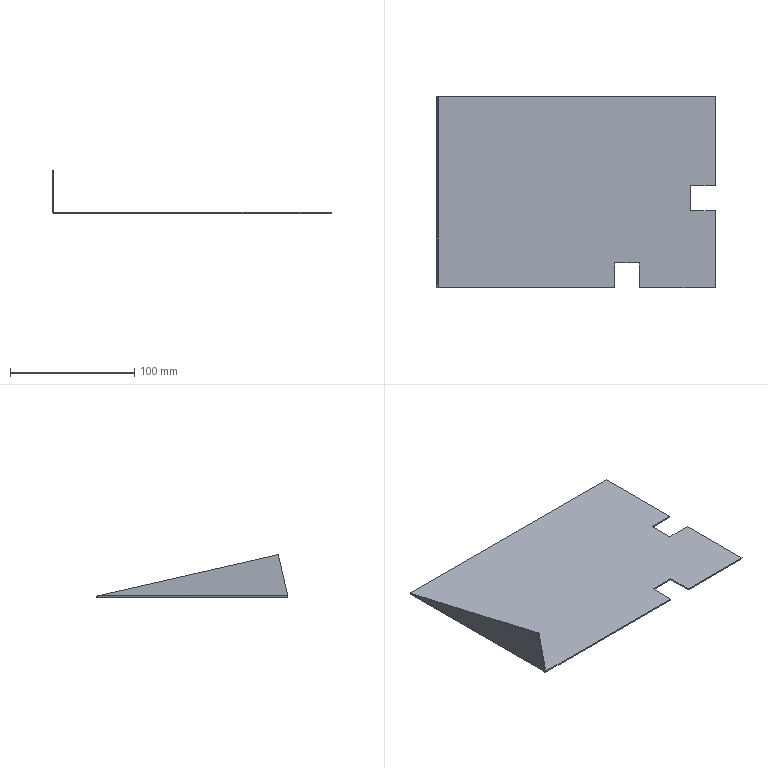Part | 1 solid | 21 faces | box 224 x 154 x 34.5 mm | volume 36229 mm3 | plane 17 | spline 2 | cylinder 2 | commonest cylinder face diameters 0.4 x1 2.4 x1
STEP:
#1=CARTESIAN_POINT('',(51.,-77.,-1.));
#2=VERTEX_POINT('',#1);
#3=CARTESIAN_POINT('',(51.,-77.,0.));
#4=VERTEX_POINT('',#3);
#5=CARTESIAN_POINT('',(51.,-77.,-1.));
#6=DIRECTION('',(0.,0.,1.));
#7=VECTOR('',#6,1000.);
#8=LINE('',#5,#7);
#9=EDGE_CURVE('',#2,#4,#8,.T.);
#10=ORIENTED_EDGE('',*,*,#9,.F.);
#11=CARTESIAN_POINT('',(112.,-77.,-1.));
#12=VERTEX_POINT('',#11);
#13=CARTESIAN_POINT('',(-112.,-77.,-1.));
#14=DIRECTION('',(1.,0.,0.));
#15=VECTOR('',#14,1000.);
#16=LINE('',#13,#15);
#17=EDGE_CURVE('',#2,#12,#16,.T.);
#18=ORIENTED_EDGE('',*,*,#17,.T.);
#19=CARTESIAN_POINT('',(112.,-77.,0.));
#20=VERTEX_POINT('',#19);
#21=CARTESIAN_POINT('',(112.,-77.,-1.));
#22=DIRECTION('',(0.,0.,1.));
#23=VECTOR('',#22,1000.);
#24=LINE('',#21,#23);
#25=EDGE_CURVE('',#12,#20,#24,.T.);
#26=ORIENTED_EDGE('',*,*,#25,.T.);
#27=CARTESIAN_POINT('',(-112.,-77.,0.));
#28=DIRECTION('',(1.,0.,0.));
#29=VECTOR('',#28,1000.);
#30=LINE('',#27,#29);
#31=EDGE_CURVE('',#4,#20,#30,.T.);
#32=ORIENTED_EDGE('',*,*,#31,.F.);
#33=EDGE_LOOP('',(#10,#18,#26,#32));
#34=FACE_OUTER_BOUND('',#33,.T.);
#35=CARTESIAN_POINT('',(-112.,-77.,-1.));
#36=DIRECTION('',(0.,-1.,0.));
#37=DIRECTION('',(0.,0.,-1.));
#38=AXIS2_PLACEMENT_3D('',#35,#36,#37);
#39=PLANE('',#38);
#40=ADVANCED_FACE('',(#34),#39,.T.);
#41=CARTESIAN_POINT('',(112.,-15.,0.));
#42=VERTEX_POINT('',#41);
#43=CARTESIAN_POINT('',(112.,-15.,-1.));
#44=VERTEX_POINT('',#43);
#45=CARTESIAN_POINT('',(112.,-15.,-1.));
#46=DIRECTION('',(0.,0.,-1.));
#47=VECTOR('',#46,1000.);
#48=LINE('',#45,#47);
#49=EDGE_CURVE('',#42,#44,#48,.T.);
#50=ORIENTED_EDGE('',*,*,#49,.F.);
#51=CARTESIAN_POINT('',(112.,77.,0.));
#52=DIRECTION('',(0.,1.,0.));
#53=VECTOR('',#52,1000.);
#54=LINE('',#51,#53);
#55=EDGE_CURVE('',#20,#42,#54,.T.);
#56=ORIENTED_EDGE('',*,*,#55,.F.);
#57=ORIENTED_EDGE('',*,*,#25,.F.);
#58=CARTESIAN_POINT('',(112.,77.,-1.));
#59=DIRECTION('',(0.,1.,0.));
#60=VECTOR('',#59,1000.);
#61=LINE('',#58,#60);
#62=EDGE_CURVE('',#12,#44,#61,.T.);
#63=ORIENTED_EDGE('',*,*,#62,.T.);
#64=EDGE_LOOP('',(#50,#56,#57,#63));
#65=FACE_OUTER_BOUND('',#64,.T.);
#66=CARTESIAN_POINT('',(112.,77.,-1.));
#67=DIRECTION('',(1.,0.,0.));
#68=DIRECTION('',(0.,1.,0.));
#69=AXIS2_PLACEMENT_3D('',#66,#67,#68);
#70=PLANE('',#69);
#71=ADVANCED_FACE('',(#65),#70,.T.);
#72=CARTESIAN_POINT('',(31.,-77.,0.));
#73=VERTEX_POINT('',#72);
#74=CARTESIAN_POINT('',(31.,-77.,-1.));
#75=VERTEX_POINT('',#74);
#76=CARTESIAN_POINT('',(31.,-77.,-1.));
#77=DIRECTION('',(0.,0.,-1.));
#78=VECTOR('',#77,1000.);
#79=LINE('',#76,#78);
#80=EDGE_CURVE('',#73,#75,#79,.T.);
#81=ORIENTED_EDGE('',*,*,#80,.F.);
#82=CARTESIAN_POINT('',(-110.8,-77.,0.));
#83=VERTEX_POINT('',#82);
#84=CARTESIAN_POINT('',(-112.,-77.,0.));
#85=DIRECTION('',(1.,0.,0.));
#86=VECTOR('',#85,1000.);
#87=LINE('',#84,#86);
#88=EDGE_CURVE('',#83,#73,#87,.T.);
#89=ORIENTED_EDGE('',*,*,#88,.F.);
#90=CARTESIAN_POINT('',(-110.8,-77.,-1.));
#91=VERTEX_POINT('',#90);
#92=CARTESIAN_POINT('',(-110.8,-77.,0.));
#93=DIRECTION('',(0.,0.,-1.));
#94=VECTOR('',#93,1000.);
#95=LINE('',#92,#94);
#96=EDGE_CURVE('',#83,#91,#95,.T.);
#97=ORIENTED_EDGE('',*,*,#96,.T.);
#98=CARTESIAN_POINT('',(-112.,-77.,-1.));
#99=DIRECTION('',(1.,0.,0.));
#100=VECTOR('',#99,1000.);
#101=LINE('',#98,#100);
#102=EDGE_CURVE('',#91,#75,#101,.T.);
#103=ORIENTED_EDGE('',*,*,#102,.T.);
#104=EDGE_LOOP('',(#81,#89,#97,#103));
#105=FACE_OUTER_BOUND('',#104,.T.);
#106=CARTESIAN_POINT('',(-112.,-77.,-1.));
#107=DIRECTION('',(0.,-1.,0.));
#108=DIRECTION('',(0.,0.,-1.));
#109=AXIS2_PLACEMENT_3D('',#106,#107,#108);
#110=PLANE('',#109);
#111=ADVANCED_FACE('',(#105),#110,.T.);
#112=ORIENTED_EDGE('',*,*,#17,.F.);
#113=CARTESIAN_POINT('',(51.,-57.,-1.));
#114=VERTEX_POINT('',#113);
#115=CARTESIAN_POINT('',(51.,0.,-1.));
#116=DIRECTION('',(0.,1.,0.));
#117=VECTOR('',#116,1000.);
#118=LINE('',#115,#117);
#119=EDGE_CURVE('',#2,#114,#118,.T.);
#120=ORIENTED_EDGE('',*,*,#119,.T.);
#121=CARTESIAN_POINT('',(31.,-57.,-1.));
#122=VERTEX_POINT('',#121);
#123=CARTESIAN_POINT('',(0.,-57.,-1.));
#124=DIRECTION('',(-1.,0.,0.));
#125=VECTOR('',#124,1000.);
#126=LINE('',#123,#125);
#127=EDGE_CURVE('',#114,#122,#126,.T.);
#128=ORIENTED_EDGE('',*,*,#127,.T.);
#129=CARTESIAN_POINT('',(31.,0.,-1.));
#130=DIRECTION('',(0.,-1.,0.));
#131=VECTOR('',#130,1000.);
#132=LINE('',#129,#131);
#133=EDGE_CURVE('',#122,#75,#132,.T.);
#134=ORIENTED_EDGE('',*,*,#133,.T.);
#135=ORIENTED_EDGE('',*,*,#102,.F.);
#136=CARTESIAN_POINT('',(-110.8,77.,-1.));
#137=VERTEX_POINT('',#136);
#138=CARTESIAN_POINT('',(-110.8,-77.,-1.));
#139=DIRECTION('',(0.,1.,0.));
#140=VECTOR('',#139,1000.);
#141=LINE('',#138,#140);
#142=EDGE_CURVE('',#91,#137,#141,.T.);
#143=ORIENTED_EDGE('',*,*,#142,.T.);
#144=CARTESIAN_POINT('',(112.,77.,-1.));
#145=VERTEX_POINT('',#144);
#146=CARTESIAN_POINT('',(-112.,77.,-1.));
#147=DIRECTION('',(-1.,0.,0.));
#148=VECTOR('',#147,1000.);
#149=LINE('',#146,#148);
#150=EDGE_CURVE('',#145,#137,#149,.T.);
#151=ORIENTED_EDGE('',*,*,#150,.F.);
#152=CARTESIAN_POINT('',(112.,5.,-1.));
#153=VERTEX_POINT('',#152);
#154=CARTESIAN_POINT('',(112.,77.,-1.));
#155=DIRECTION('',(0.,1.,0.));
#156=VECTOR('',#155,1000.);
#157=LINE('',#154,#156);
#158=EDGE_CURVE('',#153,#145,#157,.T.);
#159=ORIENTED_EDGE('',*,*,#158,.F.);
#160=CARTESIAN_POINT('',(92.,5.,-1.));
#161=VERTEX_POINT('',#160);
#162=CARTESIAN_POINT('',(0.,5.,-1.));
#163=DIRECTION('',(-1.,0.,0.));
#164=VECTOR('',#163,1000.);
#165=LINE('',#162,#164);
#166=EDGE_CURVE('',#153,#161,#165,.T.);
#167=ORIENTED_EDGE('',*,*,#166,.T.);
#168=CARTESIAN_POINT('',(92.,-15.,-1.));
#169=VERTEX_POINT('',#168);
#170=CARTESIAN_POINT('',(92.,0.,-1.));
#171=DIRECTION('',(0.,-1.,0.));
#172=VECTOR('',#171,1000.);
#173=LINE('',#170,#172);
#174=EDGE_CURVE('',#161,#169,#173,.T.);
#175=ORIENTED_EDGE('',*,*,#174,.T.);
#176=CARTESIAN_POINT('',(0.,-15.,-1.));
#177=DIRECTION('',(1.,0.,0.));
#178=VECTOR('',#177,1000.);
#179=LINE('',#176,#178);
#180=EDGE_CURVE('',#169,#44,#179,.T.);
#181=ORIENTED_EDGE('',*,*,#180,.T.);
#182=ORIENTED_EDGE('',*,*,#62,.F.);
#183=EDGE_LOOP('',(#112,#120,#128,#134,#135,#143,#151,#159,#167,#175,#181,#182));
#184=FACE_OUTER_BOUND('',#183,.T.);
#185=CARTESIAN_POINT('',(0.,0.,-1.));
#186=DIRECTION('',(0.,0.,1.));
#187=DIRECTION('',(1.,0.,0.));
#188=AXIS2_PLACEMENT_3D('',#185,#186,#187);
#189=PLANE('',#188);
#190=ADVANCED_FACE('',(#184),#189,.F.);
#191=CARTESIAN_POINT('',(51.,-57.,0.));
#192=VERTEX_POINT('',#191);
#193=CARTESIAN_POINT('',(51.,0.,0.));
#194=DIRECTION('',(0.,1.,0.));
#195=VECTOR('',#194,1000.);
#196=LINE('',#193,#195);
#197=EDGE_CURVE('',#4,#192,#196,.T.);
#198=ORIENTED_EDGE('',*,*,#197,.F.);
#199=ORIENTED_EDGE('',*,*,#31,.T.);
#200=ORIENTED_EDGE('',*,*,#55,.T.);
#201=CARTESIAN_POINT('',(92.,-15.,0.));
#202=VERTEX_POINT('',#201);
#203=CARTESIAN_POINT('',(92.,-15.,0.));
#204=DIRECTION('',(1.,0.,0.));
#205=VECTOR('',#204,1000.);
#206=LINE('',#203,#205);
#207=EDGE_CURVE('',#202,#42,#206,.T.);
#208=ORIENTED_EDGE('',*,*,#207,.F.);
#209=CARTESIAN_POINT('',(92.,5.,0.));
#210=VERTEX_POINT('',#209);
#211=CARTESIAN_POINT('',(92.,5.,0.));
#212=DIRECTION('',(0.,-1.,0.));
#213=VECTOR('',#212,1000.);
#214=LINE('',#211,#213);
#215=EDGE_CURVE('',#210,#202,#214,.T.);
#216=ORIENTED_EDGE('',*,*,#215,.F.);
#217=CARTESIAN_POINT('',(112.,5.,0.));
#218=VERTEX_POINT('',#217);
#219=CARTESIAN_POINT('',(92.,5.,0.));
#220=DIRECTION('',(-1.,0.,0.));
#221=VECTOR('',#220,1000.);
#222=LINE('',#219,#221);
#223=EDGE_CURVE('',#218,#210,#222,.T.);
#224=ORIENTED_EDGE('',*,*,#223,.F.);
#225=CARTESIAN_POINT('',(112.,77.,0.));
#226=VERTEX_POINT('',#225);
#227=CARTESIAN_POINT('',(112.,77.,0.));
#228=DIRECTION('',(0.,1.,0.));
#229=VECTOR('',#228,1000.);
#230=LINE('',#227,#229);
#231=EDGE_CURVE('',#218,#226,#230,.T.);
#232=ORIENTED_EDGE('',*,*,#231,.T.);
#233=CARTESIAN_POINT('',(-110.8,77.,0.));
#234=VERTEX_POINT('',#233);
#235=CARTESIAN_POINT('',(-112.,77.,0.));
#236=DIRECTION('',(-1.,0.,0.));
#237=VECTOR('',#236,1000.);
#238=LINE('',#235,#237);
#239=EDGE_CURVE('',#226,#234,#238,.T.);
#240=ORIENTED_EDGE('',*,*,#239,.T.);
#241=CARTESIAN_POINT('',(-110.8,-77.,0.));
#242=DIRECTION('',(0.,1.,0.));
#243=VECTOR('',#242,1000.);
#244=LINE('',#241,#243);
#245=EDGE_CURVE('',#83,#234,#244,.T.);
#246=ORIENTED_EDGE('',*,*,#245,.F.);
#247=ORIENTED_EDGE('',*,*,#88,.T.);
#248=CARTESIAN_POINT('',(31.,-57.,0.));
#249=VERTEX_POINT('',#248);
#250=CARTESIAN_POINT('',(31.,-57.,0.));
#251=DIRECTION('',(0.,-1.,0.));
#252=VECTOR('',#251,1000.);
#253=LINE('',#250,#252);
#254=EDGE_CURVE('',#249,#73,#253,.T.);
#255=ORIENTED_EDGE('',*,*,#254,.F.);
#256=CARTESIAN_POINT('',(31.,-57.,0.));
#257=DIRECTION('',(-1.,0.,0.));
#258=VECTOR('',#257,1000.);
#259=LINE('',#256,#258);
#260=EDGE_CURVE('',#192,#249,#259,.T.);
#261=ORIENTED_EDGE('',*,*,#260,.F.);
#262=EDGE_LOOP('',(#198,#199,#200,#208,#216,#224,#232,#240,#246,#247,#255,#261));
#263=FACE_OUTER_BOUND('',#262,.T.);
#264=CARTESIAN_POINT('',(0.,0.,0.));
#265=DIRECTION('',(0.,0.,1.));
#266=DIRECTION('',(1.,0.,0.));
#267=AXIS2_PLACEMENT_3D('',#264,#265,#266);
#268=PLANE('',#267);
#269=ADVANCED_FACE('',(#263),#268,.T.);
#270=CARTESIAN_POINT('',(112.,5.,-1.));
#271=DIRECTION('',(0.,0.,1.));
#272=VECTOR('',#271,1000.);
#273=LINE('',#270,#272);
#274=EDGE_CURVE('',#153,#218,#273,.T.);
#275=ORIENTED_EDGE('',*,*,#274,.F.);
#276=ORIENTED_EDGE('',*,*,#158,.T.);
#277=CARTESIAN_POINT('',(112.,77.,-1.));
#278=DIRECTION('',(0.,0.,1.));
#279=VECTOR('',#278,1000.);
#280=LINE('',#277,#279);
#281=EDGE_CURVE('',#145,#226,#280,.T.);
#282=ORIENTED_EDGE('',*,*,#281,.T.);
#283=ORIENTED_EDGE('',*,*,#231,.F.);
#284=EDGE_LOOP('',(#275,#276,#282,#283));
#285=FACE_OUTER_BOUND('',#284,.T.);
#286=CARTESIAN_POINT('',(112.,77.,-1.));
#287=DIRECTION('',(1.,0.,0.));
#288=DIRECTION('',(0.,1.,0.));
#289=AXIS2_PLACEMENT_3D('',#286,#287,#288);
#290=PLANE('',#289);
#291=ADVANCED_FACE('',(#285),#290,.T.);
#292=CARTESIAN_POINT('',(-110.8,77.,0.));
#293=DIRECTION('',(0.,0.,-1.));
#294=VECTOR('',#293,1000.);
#295=LINE('',#292,#294);
#296=EDGE_CURVE('',#234,#137,#295,.T.);
#297=ORIENTED_EDGE('',*,*,#296,.F.);
#298=ORIENTED_EDGE('',*,*,#239,.F.);
#299=ORIENTED_EDGE('',*,*,#281,.F.);
#300=ORIENTED_EDGE('',*,*,#150,.T.);
#301=EDGE_LOOP('',(#297,#298,#299,#300));
#302=FACE_OUTER_BOUND('',#301,.T.);
#303=CARTESIAN_POINT('',(-112.,77.,-1.));
#304=DIRECTION('',(0.,1.,0.));
#305=DIRECTION('',(0.,0.,1.));
#306=AXIS2_PLACEMENT_3D('',#303,#304,#305);
#307=PLANE('',#306);
#308=ADVANCED_FACE('',(#302),#307,.T.);
#309=CARTESIAN_POINT('',(-111.,76.126,0.2));
#310=VERTEX_POINT('',#309);
#311=CARTESIAN_POINT('',(-112.,76.126,0.2));
#312=VERTEX_POINT('',#311);
#313=CARTESIAN_POINT('',(-112.,76.126,0.2));
#314=DIRECTION('',(-1.,0.,0.));
#315=VECTOR('',#314,1000.);
#316=LINE('',#313,#315);
#317=EDGE_CURVE('',#310,#312,#316,.T.);
#318=ORIENTED_EDGE('',*,*,#317,.F.);
#319=CARTESIAN_POINT('',(-110.8,77.,0.));
#320=CARTESIAN_POINT('',(-110.852,76.854,0.));
#321=CARTESIAN_POINT('',(-110.904,76.709,0.02155));
#322=CARTESIAN_POINT('',(-110.978,76.418,0.0956));
#323=CARTESIAN_POINT('',(-111.,76.272,0.1476));
#324=CARTESIAN_POINT('',(-111.,76.126,0.2));
#325=B_SPLINE_CURVE_WITH_KNOTS('',3,(#319,#320,#321,#322,#323,#324),.UNSPECIFIED.,.F.,.F.,(4,2,4),(0.,0.5,1.),.UNSPECIFIED.);
#326=EDGE_CURVE('',#234,#310,#325,.T.);
#327=ORIENTED_EDGE('',*,*,#326,.F.);
#328=ORIENTED_EDGE('',*,*,#296,.T.);
#329=CARTESIAN_POINT('',(-110.8,77.,-1.));
#330=CARTESIAN_POINT('',(-110.959,76.927,-1.));
#331=CARTESIAN_POINT('',(-111.112,76.855,-0.9694));
#332=CARTESIAN_POINT('',(-111.405,76.708,-0.8482));
#333=CARTESIAN_POINT('',(-111.537,76.637,-0.7605));
#334=CARTESIAN_POINT('',(-111.76,76.49,-0.5371));
#335=CARTESIAN_POINT('',(-111.848,76.418,-0.4051));
#336=CARTESIAN_POINT('',(-111.969,76.272,-0.1139));
#337=CARTESIAN_POINT('',(-112.,76.2,0.04144));
#338=CARTESIAN_POINT('',(-112.,76.126,0.2));
#339=B_SPLINE_CURVE_WITH_KNOTS('',3,(#329,#330,#331,#332,#333,#334,#335,#336,#337,#338),.UNSPECIFIED.,.F.,.F.,(4,2,2,2,4),(0.,0.0005161,0.001032,0.001548,0.002065),.UNSPECIFIED.);
#340=EDGE_CURVE('',#137,#312,#339,.T.);
#341=ORIENTED_EDGE('',*,*,#340,.T.);
#342=EDGE_LOOP('',(#318,#327,#328,#341));
#343=FACE_OUTER_BOUND('',#342,.T.);
#344=CARTESIAN_POINT('',(-110.8,77.,-1.01));
#345=CARTESIAN_POINT('',(-110.958,76.927,-1.01));
#346=CARTESIAN_POINT('',(-111.117,76.854,-0.9785));
#347=CARTESIAN_POINT('',(-111.409,76.709,-0.8573));
#348=CARTESIAN_POINT('',(-111.544,76.636,-0.7676));
#349=CARTESIAN_POINT('',(-111.768,76.49,-0.5436));
#350=CARTESIAN_POINT('',(-111.857,76.418,-0.4094));
#351=CARTESIAN_POINT('',(-111.979,76.272,-0.1167));
#352=CARTESIAN_POINT('',(-112.01,76.199,0.04159));
#353=CARTESIAN_POINT('',(-112.01,76.126,0.2));
#354=CARTESIAN_POINT('',(-110.8,77.,-1.));
#355=CARTESIAN_POINT('',(-110.957,76.927,-1.));
#356=CARTESIAN_POINT('',(-111.114,76.854,-0.9688));
#357=CARTESIAN_POINT('',(-111.404,76.709,-0.8485));
#358=CARTESIAN_POINT('',(-111.537,76.636,-0.7596));
#359=CARTESIAN_POINT('',(-111.76,76.49,-0.5375));
#360=CARTESIAN_POINT('',(-111.849,76.418,-0.4043));
#361=CARTESIAN_POINT('',(-111.969,76.272,-0.1141));
#362=CARTESIAN_POINT('',(-112.,76.199,0.0429));
#363=CARTESIAN_POINT('',(-112.,76.126,0.2));
#364=CARTESIAN_POINT('',(-110.8,77.,0.));
#365=CARTESIAN_POINT('',(-110.826,76.927,0.));
#366=CARTESIAN_POINT('',(-110.852,76.854,0.005205));
#367=CARTESIAN_POINT('',(-110.901,76.709,0.02524));
#368=CARTESIAN_POINT('',(-110.923,76.636,0.04007));
#369=CARTESIAN_POINT('',(-110.96,76.49,0.07709));
#370=CARTESIAN_POINT('',(-110.975,76.418,0.09928));
#371=CARTESIAN_POINT('',(-110.995,76.272,0.1477));
#372=CARTESIAN_POINT('',(-111.,76.199,0.1738));
#373=CARTESIAN_POINT('',(-111.,76.126,0.2));
#374=CARTESIAN_POINT('',(-110.8,77.,0.0101));
#375=CARTESIAN_POINT('',(-110.825,76.927,0.0101));
#376=CARTESIAN_POINT('',(-110.85,76.854,0.01504));
#377=CARTESIAN_POINT('',(-110.896,76.709,0.03407));
#378=CARTESIAN_POINT('',(-110.917,76.636,0.04814));
#379=CARTESIAN_POINT('',(-110.952,76.49,0.0833));
#380=CARTESIAN_POINT('',(-110.966,76.418,0.1044));
#381=CARTESIAN_POINT('',(-110.985,76.272,0.1503));
#382=CARTESIAN_POINT('',(-110.99,76.199,0.1751));
#383=CARTESIAN_POINT('',(-110.99,76.126,0.2));
#384=B_SPLINE_SURFACE_WITH_KNOTS('',1,3,((#344,#345,#346,#347,#348,#349,#350,#351,#352,#353),(#354,#355,#356,#357,#358,#359,#360,#361,#362,#363),(#364,#365,#366,#367,#368,#369,#370,#371,#372,#373),(#374,#375,#376,#377,#378,#379,#380,#381,#382,#383)),.UNSPECIFIED.,.F.,.F.,.F.,(2,1,1,2),(4,2,2,2,4),(-0.01,0.,1.,1.01),(0.,0.25,0.5,0.75,1.),.UNSPECIFIED.);
#385=ADVANCED_FACE('',(#343),#384,.F.);
#386=CARTESIAN_POINT('',(-111.,-76.954,0.2));
#387=VERTEX_POINT('',#386);
#388=CARTESIAN_POINT('',(-111.,-76.954,0.2));
#389=CARTESIAN_POINT('',(-111.,-76.962,0.1476));
#390=CARTESIAN_POINT('',(-110.978,-76.969,0.0956));
#391=CARTESIAN_POINT('',(-110.904,-76.985,0.02155));
#392=CARTESIAN_POINT('',(-110.852,-76.992,0.));
#393=CARTESIAN_POINT('',(-110.8,-77.,0.));
#394=B_SPLINE_CURVE_WITH_KNOTS('',3,(#388,#389,#390,#391,#392,#393),.UNSPECIFIED.,.F.,.F.,(4,2,4),(0.,0.5,1.),.UNSPECIFIED.);
#395=EDGE_CURVE('',#387,#83,#394,.T.);
#396=ORIENTED_EDGE('',*,*,#395,.F.);
#397=CARTESIAN_POINT('',(-112.,-76.954,0.2));
#398=VERTEX_POINT('',#397);
#399=CARTESIAN_POINT('',(-111.,-76.954,0.2));
#400=DIRECTION('',(-1.,0.,0.));
#401=VECTOR('',#400,1000.);
#402=LINE('',#399,#401);
#403=EDGE_CURVE('',#387,#398,#402,.T.);
#404=ORIENTED_EDGE('',*,*,#403,.T.);
#405=CARTESIAN_POINT('',(-112.,-76.954,0.2));
#406=CARTESIAN_POINT('',(-112.,-76.958,0.04292));
#407=CARTESIAN_POINT('',(-111.969,-76.962,-0.1141));
#408=CARTESIAN_POINT('',(-111.849,-76.969,-0.4043));
#409=CARTESIAN_POINT('',(-111.76,-76.973,-0.5375));
#410=CARTESIAN_POINT('',(-111.537,-76.981,-0.7596));
#411=CARTESIAN_POINT('',(-111.404,-76.985,-0.8485));
#412=CARTESIAN_POINT('',(-111.114,-76.992,-0.9688));
#413=CARTESIAN_POINT('',(-110.957,-76.996,-1.));
#414=CARTESIAN_POINT('',(-110.8,-77.,-1.));
#415=B_SPLINE_CURVE_WITH_KNOTS('',3,(#405,#406,#407,#408,#409,#410,#411,#412,#413,#414),.UNSPECIFIED.,.F.,.F.,(4,2,2,2,4),(0.,0.25,0.5,0.75,1.),.UNSPECIFIED.);
#416=EDGE_CURVE('',#398,#91,#415,.T.);
#417=ORIENTED_EDGE('',*,*,#416,.T.);
#418=ORIENTED_EDGE('',*,*,#96,.F.);
#419=EDGE_LOOP('',(#396,#404,#417,#418));
#420=FACE_OUTER_BOUND('',#419,.T.);
#421=CARTESIAN_POINT('',(-112.01,-76.954,0.2));
#422=CARTESIAN_POINT('',(-112.01,-76.958,0.04158));
#423=CARTESIAN_POINT('',(-111.979,-76.962,-0.1167));
#424=CARTESIAN_POINT('',(-111.857,-76.969,-0.4094));
#425=CARTESIAN_POINT('',(-111.768,-76.973,-0.5436));
#426=CARTESIAN_POINT('',(-111.544,-76.981,-0.7676));
#427=CARTESIAN_POINT('',(-111.409,-76.985,-0.8573));
#428=CARTESIAN_POINT('',(-111.117,-76.992,-0.9785));
#429=CARTESIAN_POINT('',(-110.958,-76.996,-1.01));
#430=CARTESIAN_POINT('',(-110.8,-77.,-1.01));
#431=CARTESIAN_POINT('',(-112.,-76.954,0.2));
#432=CARTESIAN_POINT('',(-112.,-76.958,0.04289));
#433=CARTESIAN_POINT('',(-111.969,-76.962,-0.1141));
#434=CARTESIAN_POINT('',(-111.849,-76.969,-0.4043));
#435=CARTESIAN_POINT('',(-111.76,-76.973,-0.5375));
#436=CARTESIAN_POINT('',(-111.537,-76.981,-0.7596));
#437=CARTESIAN_POINT('',(-111.404,-76.985,-0.8485));
#438=CARTESIAN_POINT('',(-111.114,-76.992,-0.9688));
#439=CARTESIAN_POINT('',(-110.957,-76.996,-1.));
#440=CARTESIAN_POINT('',(-110.8,-77.,-1.));
#441=CARTESIAN_POINT('',(-111.,-76.954,0.2));
#442=CARTESIAN_POINT('',(-111.,-76.958,0.1738));
#443=CARTESIAN_POINT('',(-110.995,-76.962,0.1477));
#444=CARTESIAN_POINT('',(-110.975,-76.969,0.09928));
#445=CARTESIAN_POINT('',(-110.96,-76.973,0.07709));
#446=CARTESIAN_POINT('',(-110.923,-76.981,0.04007));
#447=CARTESIAN_POINT('',(-110.901,-76.985,0.02524));
#448=CARTESIAN_POINT('',(-110.852,-76.992,0.005205));
#449=CARTESIAN_POINT('',(-110.826,-76.996,0.));
#450=CARTESIAN_POINT('',(-110.8,-77.,0.));
#451=CARTESIAN_POINT('',(-110.99,-76.954,0.2));
#452=CARTESIAN_POINT('',(-110.99,-76.958,0.1751));
#453=CARTESIAN_POINT('',(-110.985,-76.962,0.1503));
#454=CARTESIAN_POINT('',(-110.966,-76.969,0.1044));
#455=CARTESIAN_POINT('',(-110.952,-76.973,0.0833));
#456=CARTESIAN_POINT('',(-110.917,-76.981,0.04814));
#457=CARTESIAN_POINT('',(-110.896,-76.985,0.03407));
#458=CARTESIAN_POINT('',(-110.85,-76.992,0.01504));
#459=CARTESIAN_POINT('',(-110.825,-76.996,0.0101));
#460=CARTESIAN_POINT('',(-110.8,-77.,0.0101));
#461=B_SPLINE_SURFACE_WITH_KNOTS('',1,3,((#421,#422,#423,#424,#425,#426,#427,#428,#429,#430),(#431,#432,#433,#434,#435,#436,#437,#438,#439,#440),(#441,#442,#443,#444,#445,#446,#447,#448,#449,#450),(#451,#452,#453,#454,#455,#456,#457,#458,#459,#460)),.UNSPECIFIED.,.F.,.F.,.F.,(2,1,1,2),(4,2,2,2,4),(-0.01,0.,1.,1.01),(0.,0.25,0.5,0.75,1.),.UNSPECIFIED.);
#462=ADVANCED_FACE('',(#420),#461,.F.);
#463=ORIENTED_EDGE('',*,*,#142,.F.);
#464=ORIENTED_EDGE('',*,*,#416,.F.);
#465=CARTESIAN_POINT('',(-112.,76.126,0.2));
#466=DIRECTION('',(0.,1.,0.));
#467=VECTOR('',#466,1000.);
#468=LINE('',#465,#467);
#469=EDGE_CURVE('',#398,#312,#468,.T.);
#470=ORIENTED_EDGE('',*,*,#469,.T.);
#471=ORIENTED_EDGE('',*,*,#340,.F.);
#472=EDGE_LOOP('',(#463,#464,#470,#471));
#473=FACE_OUTER_BOUND('',#472,.T.);
#474=CARTESIAN_POINT('',(-110.8,-77.,0.2));
#475=DIRECTION('',(0.,-1.,0.));
#476=DIRECTION('',(-1.,0.,0.));
#477=AXIS2_PLACEMENT_3D('',#474,#475,#476);
#478=CYLINDRICAL_SURFACE('',#477,1.2);
#479=ADVANCED_FACE('',(#473),#478,.T.);
#480=ORIENTED_EDGE('',*,*,#245,.T.);
#481=ORIENTED_EDGE('',*,*,#326,.T.);
#482=CARTESIAN_POINT('',(-111.,76.126,0.2));
#483=DIRECTION('',(0.,-1.,0.));
#484=VECTOR('',#483,1000.);
#485=LINE('',#482,#484);
#486=EDGE_CURVE('',#310,#387,#485,.T.);
#487=ORIENTED_EDGE('',*,*,#486,.T.);
#488=ORIENTED_EDGE('',*,*,#395,.T.);
#489=EDGE_LOOP('',(#480,#481,#487,#488));
#490=FACE_OUTER_BOUND('',#489,.T.);
#491=CARTESIAN_POINT('',(-110.8,-77.,0.2));
#492=DIRECTION('',(0.,-1.,0.));
#493=DIRECTION('',(-1.,0.,0.));
#494=AXIS2_PLACEMENT_3D('',#491,#492,#493);
#495=CYLINDRICAL_SURFACE('',#494,0.2);
#496=ADVANCED_FACE('',(#490),#495,.F.);
#497=ORIENTED_EDGE('',*,*,#317,.T.);
#498=CARTESIAN_POINT('',(-112.,-69.331,33.5));
#499=VERTEX_POINT('',#498);
#500=CARTESIAN_POINT('',(-112.,3.835,16.75));
#501=DIRECTION('',(0.,0.9748,-0.2232));
#502=VECTOR('',#501,1000.);
#503=LINE('',#500,#502);
#504=EDGE_CURVE('',#499,#312,#503,.T.);
#505=ORIENTED_EDGE('',*,*,#504,.F.);
#506=CARTESIAN_POINT('',(-111.,-69.331,33.5));
#507=VERTEX_POINT('',#506);
#508=CARTESIAN_POINT('',(-112.,-69.331,33.5));
#509=DIRECTION('',(1.,0.,0.));
#510=VECTOR('',#509,1000.);
#511=LINE('',#508,#510);
#512=EDGE_CURVE('',#499,#507,#511,.T.);
#513=ORIENTED_EDGE('',*,*,#512,.T.);
#514=CARTESIAN_POINT('',(-111.,-69.331,33.5));
#515=DIRECTION('',(0.,0.9748,-0.2232));
#516=VECTOR('',#515,1000.);
#517=LINE('',#514,#516);
#518=EDGE_CURVE('',#507,#310,#517,.T.);
#519=ORIENTED_EDGE('',*,*,#518,.T.);
#520=EDGE_LOOP('',(#497,#505,#513,#519));
#521=FACE_OUTER_BOUND('',#520,.T.);
#522=CARTESIAN_POINT('',(-112.,-69.331,33.5));
#523=DIRECTION('',(0.,-0.2232,-0.9748));
#524=DIRECTION('',(0.,0.9748,-0.2232));
#525=AXIS2_PLACEMENT_3D('',#522,#523,#524);
#526=PLANE('',#525);
#527=ADVANCED_FACE('',(#521),#526,.F.);
#528=ORIENTED_EDGE('',*,*,#403,.F.);
#529=CARTESIAN_POINT('',(-111.,-77.,0.));
#530=DIRECTION('',(0.,0.2232,0.9748));
#531=VECTOR('',#530,1000.);
#532=LINE('',#529,#531);
#533=EDGE_CURVE('',#387,#507,#532,.T.);
#534=ORIENTED_EDGE('',*,*,#533,.T.);
#535=ORIENTED_EDGE('',*,*,#512,.F.);
#536=CARTESIAN_POINT('',(-112.,-73.165,16.75));
#537=DIRECTION('',(0.,0.2232,0.9748));
#538=VECTOR('',#537,1000.);
#539=LINE('',#536,#538);
#540=EDGE_CURVE('',#398,#499,#539,.T.);
#541=ORIENTED_EDGE('',*,*,#540,.F.);
#542=EDGE_LOOP('',(#528,#534,#535,#541));
#543=FACE_OUTER_BOUND('',#542,.T.);
#544=CARTESIAN_POINT('',(-112.,-77.,0.));
#545=DIRECTION('',(0.,0.9748,-0.2232));
#546=DIRECTION('',(0.,0.2232,0.9748));
#547=AXIS2_PLACEMENT_3D('',#544,#545,#546);
#548=PLANE('',#547);
#549=ADVANCED_FACE('',(#543),#548,.F.);
#550=ORIENTED_EDGE('',*,*,#469,.F.);
#551=ORIENTED_EDGE('',*,*,#540,.T.);
#552=ORIENTED_EDGE('',*,*,#504,.T.);
#553=EDGE_LOOP('',(#550,#551,#552));
#554=FACE_OUTER_BOUND('',#553,.T.);
#555=CARTESIAN_POINT('',(-112.,0.,0.));
#556=DIRECTION('',(1.,0.,0.));
#557=DIRECTION('',(0.,0.,-1.));
#558=AXIS2_PLACEMENT_3D('',#555,#556,#557);
#559=PLANE('',#558);
#560=ADVANCED_FACE('',(#554),#559,.F.);
#561=ORIENTED_EDGE('',*,*,#533,.F.);
#562=ORIENTED_EDGE('',*,*,#486,.F.);
#563=ORIENTED_EDGE('',*,*,#518,.F.);
#564=EDGE_LOOP('',(#561,#562,#563));
#565=FACE_OUTER_BOUND('',#564,.T.);
#566=CARTESIAN_POINT('',(-111.,0.,0.));
#567=DIRECTION('',(1.,0.,0.));
#568=DIRECTION('',(0.,0.,-1.));
#569=AXIS2_PLACEMENT_3D('',#566,#567,#568);
#570=PLANE('',#569);
#571=ADVANCED_FACE('',(#565),#570,.T.);
#572=CARTESIAN_POINT('',(92.,5.,-10.));
#573=DIRECTION('',(0.,0.,1.));
#574=VECTOR('',#573,1000.);
#575=LINE('',#572,#574);
#576=EDGE_CURVE('',#161,#210,#575,.T.);
#577=ORIENTED_EDGE('',*,*,#576,.T.);
#578=ORIENTED_EDGE('',*,*,#215,.T.);
#579=CARTESIAN_POINT('',(92.,-15.,-10.));
#580=DIRECTION('',(0.,0.,1.));
#581=VECTOR('',#580,1000.);
#582=LINE('',#579,#581);
#583=EDGE_CURVE('',#169,#202,#582,.T.);
#584=ORIENTED_EDGE('',*,*,#583,.F.);
#585=ORIENTED_EDGE('',*,*,#174,.F.);
#586=EDGE_LOOP('',(#577,#578,#584,#585));
#587=FACE_OUTER_BOUND('',#586,.T.);
#588=CARTESIAN_POINT('',(92.,5.,-10.));
#589=DIRECTION('',(-1.,0.,0.));
#590=DIRECTION('',(0.,-1.,0.));
#591=AXIS2_PLACEMENT_3D('',#588,#589,#590);
#592=PLANE('',#591);
#593=ADVANCED_FACE('',(#587),#592,.F.);
#594=ORIENTED_EDGE('',*,*,#583,.T.);
#595=ORIENTED_EDGE('',*,*,#207,.T.);
#596=ORIENTED_EDGE('',*,*,#49,.T.);
#597=ORIENTED_EDGE('',*,*,#180,.F.);
#598=EDGE_LOOP('',(#594,#595,#596,#597));
#599=FACE_OUTER_BOUND('',#598,.T.);
#600=CARTESIAN_POINT('',(92.,-15.,-10.));
#601=DIRECTION('',(0.,-1.,0.));
#602=DIRECTION('',(0.,0.,-1.));
#603=AXIS2_PLACEMENT_3D('',#600,#601,#602);
#604=PLANE('',#603);
#605=ADVANCED_FACE('',(#599),#604,.F.);
#606=ORIENTED_EDGE('',*,*,#274,.T.);
#607=ORIENTED_EDGE('',*,*,#223,.T.);
#608=ORIENTED_EDGE('',*,*,#576,.F.);
#609=ORIENTED_EDGE('',*,*,#166,.F.);
#610=EDGE_LOOP('',(#606,#607,#608,#609));
#611=FACE_OUTER_BOUND('',#610,.T.);
#612=CARTESIAN_POINT('',(92.,5.,-10.));
#613=DIRECTION('',(0.,1.,0.));
#614=DIRECTION('',(0.,0.,1.));
#615=AXIS2_PLACEMENT_3D('',#612,#613,#614);
#616=PLANE('',#615);
#617=ADVANCED_FACE('',(#611),#616,.F.);
#618=CARTESIAN_POINT('',(51.,-57.,-10.));
#619=DIRECTION('',(0.,0.,1.));
#620=VECTOR('',#619,1000.);
#621=LINE('',#618,#620);
#622=EDGE_CURVE('',#114,#192,#621,.T.);
#623=ORIENTED_EDGE('',*,*,#622,.T.);
#624=ORIENTED_EDGE('',*,*,#260,.T.);
#625=CARTESIAN_POINT('',(31.,-57.,-10.));
#626=DIRECTION('',(0.,0.,1.));
#627=VECTOR('',#626,1000.);
#628=LINE('',#625,#627);
#629=EDGE_CURVE('',#122,#249,#628,.T.);
#630=ORIENTED_EDGE('',*,*,#629,.F.);
#631=ORIENTED_EDGE('',*,*,#127,.F.);
#632=EDGE_LOOP('',(#623,#624,#630,#631));
#633=FACE_OUTER_BOUND('',#632,.T.);
#634=CARTESIAN_POINT('',(31.,-57.,-10.));
#635=DIRECTION('',(0.,1.,0.));
#636=DIRECTION('',(0.,0.,1.));
#637=AXIS2_PLACEMENT_3D('',#634,#635,#636);
#638=PLANE('',#637);
#639=ADVANCED_FACE('',(#633),#638,.F.);
#640=ORIENTED_EDGE('',*,*,#9,.T.);
#641=ORIENTED_EDGE('',*,*,#197,.T.);
#642=ORIENTED_EDGE('',*,*,#622,.F.);
#643=ORIENTED_EDGE('',*,*,#119,.F.);
#644=EDGE_LOOP('',(#640,#641,#642,#643));
#645=FACE_OUTER_BOUND('',#644,.T.);
#646=CARTESIAN_POINT('',(51.,-57.,-10.));
#647=DIRECTION('',(1.,0.,0.));
#648=DIRECTION('',(0.,0.,-1.));
#649=AXIS2_PLACEMENT_3D('',#646,#647,#648);
#650=PLANE('',#649);
#651=ADVANCED_FACE('',(#645),#650,.F.);
#652=ORIENTED_EDGE('',*,*,#80,.T.);
#653=ORIENTED_EDGE('',*,*,#133,.F.);
#654=ORIENTED_EDGE('',*,*,#629,.T.);
#655=ORIENTED_EDGE('',*,*,#254,.T.);
#656=EDGE_LOOP('',(#652,#653,#654,#655));
#657=FACE_OUTER_BOUND('',#656,.T.);
#658=CARTESIAN_POINT('',(31.,-57.,-10.));
#659=DIRECTION('',(-1.,0.,0.));
#660=DIRECTION('',(0.,-1.,0.));
#661=AXIS2_PLACEMENT_3D('',#658,#659,#660);
#662=PLANE('',#661);
#663=ADVANCED_FACE('',(#657),#662,.F.);
#664=CLOSED_SHELL('',(#40,#71,#111,#190,#269,#291,#308,#385,#462,#479,#496,#527,#549,#560,#571,#593,#605,#617,#639,#651,#663));
#665=MANIFOLD_SOLID_BREP('',#664);
#666=CARTESIAN_POINT('',(0.,0.,0.));
#667=DIRECTION('',(0.,0.,1.));
#668=DIRECTION('',(1.,0.,0.));
#669=AXIS2_PLACEMENT_3D('',#666,#667,#668);
#670=(LENGTH_UNIT()NAMED_UNIT(*)SI_UNIT(.MILLI.,.METRE.));
#671=UNCERTAINTY_MEASURE_WITH_UNIT(LENGTH_MEASURE(0.00001),#670,'','');
#672=(NAMED_UNIT(*)PLANE_ANGLE_UNIT()SI_UNIT($,.RADIAN.));
#673=(NAMED_UNIT(*)SI_UNIT($,.STERADIAN.)SOLID_ANGLE_UNIT());
#674=(GEOMETRIC_REPRESENTATION_CONTEXT(3)GLOBAL_UNCERTAINTY_ASSIGNED_CONTEXT((#671))GLOBAL_UNIT_ASSIGNED_CONTEXT((#670,#672,#673))REPRESENTATION_CONTEXT('',''));
#675=ADVANCED_BREP_SHAPE_REPRESENTATION('',(#665,#669),#674);